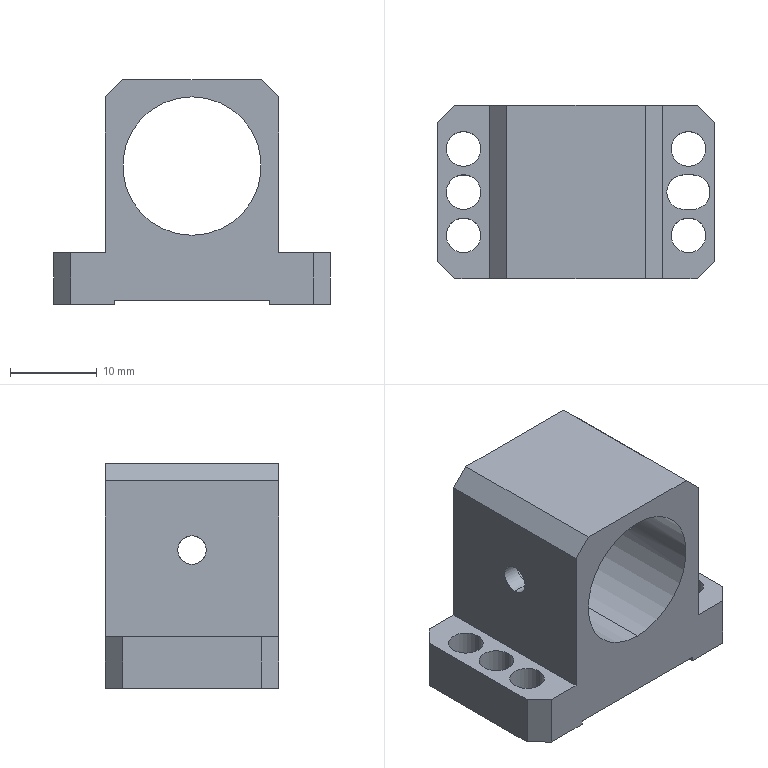NC program | NX | posted with a generic post | part box 32 x 20 x 26 mm
Lines 1 to 231 of 2499:
N10 G17 G21 G94 G90
(FLOOR_WALL_COPY , TOOL : D10JING)
N12 T11 M6
N14 G54
N16 G17 G0 G90 X17.997 Y20. B0. C0. S9500 M3
N18 G43 Z30. H11
N20 Z6.5
N22 G94 G1 Z3.5 F1250.
N24 Y17.
N26 Y-17.
N28 X13.426
N30 Y17.
N32 X8.855
N34 Y-17.
N36 X4.284
N38 Y17.
N40 X-0.287
N42 Y-17.
N44 X-4.858
N46 Y17.
N48 X-9.429
N50 Y-17.
N52 X-14.
N54 Y17.
N56 Y20.
N58 Z6.5
N60 G0 Z30.
N62 X17.997
N64 Z6.
N66 G1 Z3.
N68 Y17.
N70 Y-17.
N72 X13.426
N74 Y17.
N76 X8.855
N78 Y-17.
N80 X4.284
N82 Y17.
N84 X-0.287
N86 Y-17.
N88 X-4.858
N90 Y17.
N92 X-9.429
N94 Y-17.
N96 X-14.
N98 Y17.
N100 Y20.
N102 Z6.
N104 G0 Z30.
N106 X17.997
N108 Z5.5
N110 G1 Z2.5
N112 Y17.
N114 Y-17.
N116 X13.426
N118 Y17.
N120 X8.855
N122 Y-17.
N124 X4.284
N126 Y17.
N128 X-0.287
N130 Y-17.
N132 X-4.858
N134 Y17.
N136 X-9.429
N138 Y-17.
N140 X-14.
N142 Y17.
N144 Y20.
N146 Z5.5
N148 G0 Z30.
N150 X17.997
N152 Z5.
N154 G1 Z2.
N156 Y17.
N158 Y-17.
N160 X13.426
N162 Y17.
N164 X8.855
N166 Y-17.
N168 X4.284
N170 Y17.
N172 X-0.287
N174 Y-17.
N176 X-4.858
N178 Y17.
N180 X-9.429
N182 Y-17.
N184 X-14.
N186 Y17.
N188 Y20.
N190 Z5.
N192 G0 Z30.
N194 X17.997
N196 Z4.5
N198 G1 Z1.5
N200 Y17.
N202 Y-17.
N204 X13.426
N206 Y17.
N208 X8.855
N210 Y-17.
N212 X4.284
N214 Y17.
N216 X-0.287
N218 Y-17.
N220 X-4.858
N222 Y17.
N224 X-9.429
N226 Y-17.
N228 X-14.
N230 Y17.
N232 Y20.
N234 Z4.5
N236 G0 Z30.
N238 X17.997
N240 Z4.
N242 G1 Z1.
N244 Y17.
N246 Y-17.
N248 X13.426
N250 Y17.
N252 X8.855
N254 Y-17.
N256 X4.284
N258 Y17.
N260 X-0.287
N262 Y-17.
N264 X-4.858
N266 Y17.
N268 X-9.429
N270 Y-17.
N272 X-14.
N274 Y17.
N276 Y20.
N278 Z4.
N280 G0 Z30.
N282 X17.997
N284 Z3.5
N286 G1 Z0.5
N288 Y17.
N290 Y-17.
N292 X13.426
N294 Y17.
N296 X8.855
N298 Y-17.
N300 X4.284
N302 Y17.
N304 X-0.287
N306 Y-17.
N308 X-4.858
N310 Y17.
N312 X-9.429
N314 Y-17.
N316 X-14.
N318 Y17.
N320 Y20.
N322 Z3.5
N324 G0 Z30.
N326 X17.997
N328 Z3.
N330 G1 Z0.
N332 Y17.
N334 Y-17.
N336 X13.426
N338 Y17.
N340 X8.855
N342 Y-17.
N344 X4.284
N346 Y17.
N348 X-0.287
N350 Y-17.
N352 X-4.858
N354 Y17.
N356 X-9.429
N358 Y-17.
N360 X-14.
N362 Y17.
N364 Y20.
N366 Z3.
N368 G0 Z30.
(FLOOR_WALL_COPY_COPY , TOOL : D10JING)
N370 X3.997 Y18.
N372 Z2.5
N374 G1 Z-0.5
N376 Y15.
N378 Y-15.
N380 X-0.001
N382 Y15.
N384 X-4.
N386 Y-15.
N388 Y-18.
N390 Z2.5
N392 G0 Z30.
N394 M5
(DRILLING , TOOL : D6A45)
N396 T07 M6
N398 G54
N400 G17 G0 G90 X13. Y-5. B0. C0. S5000 M3
N402 G43 Z30. H7
N404 G94 G81 G98 Z-1. F250. R3.
N406 X12.5 Y0.
N408 X13. Y5.
N410 X-13.
N412 Y0.
N414 Y-5.
N416 G80
N418 G0 X-13. Y-5. Z30.
N420 M5
(DRILLING_COPY , TOOL : 4.0ZT)
N422 T14 M6
N424 G54
N426 G17 G0 G90 X-13. Y5. B0. C0. S2000 M3
N428 G43 Z30. H14
N430 G94 G83 G98 Z-8.702 F250. Q2. R3.
N432 Y-5.
N434 X13.
N436 Y5.
N438 G80
N440 G0 X13. Y5. Z30.
N442 M5